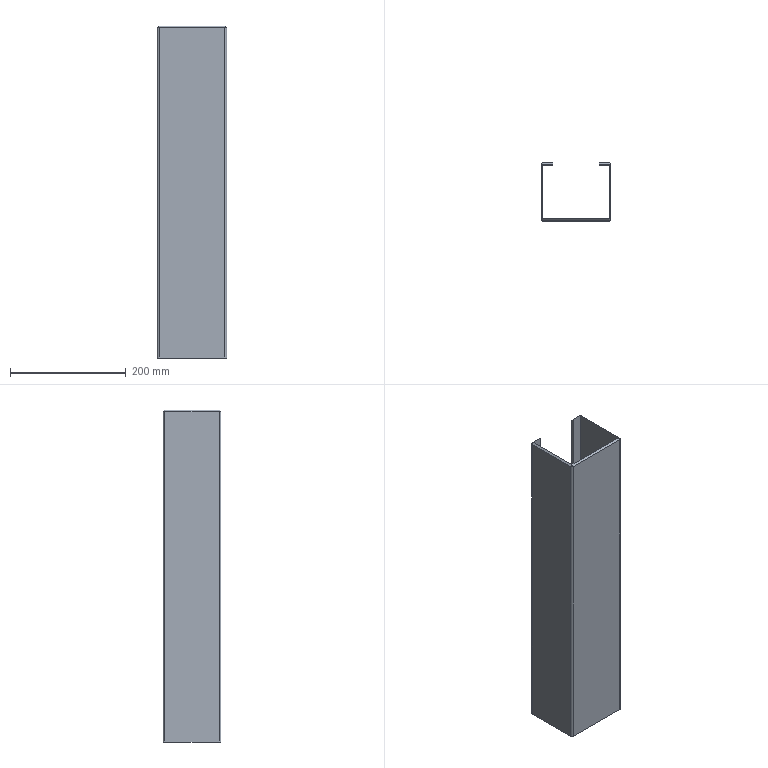Part | STEP file | TS-010-01 | 1 solid | 54 faces | box 120 x 100 x 572.5 mm | volume 586310 mm3 | plane 42 | cylinder 8 | cone 4 | commonest cylinder face diameters 0.4 x4 6.4 x4